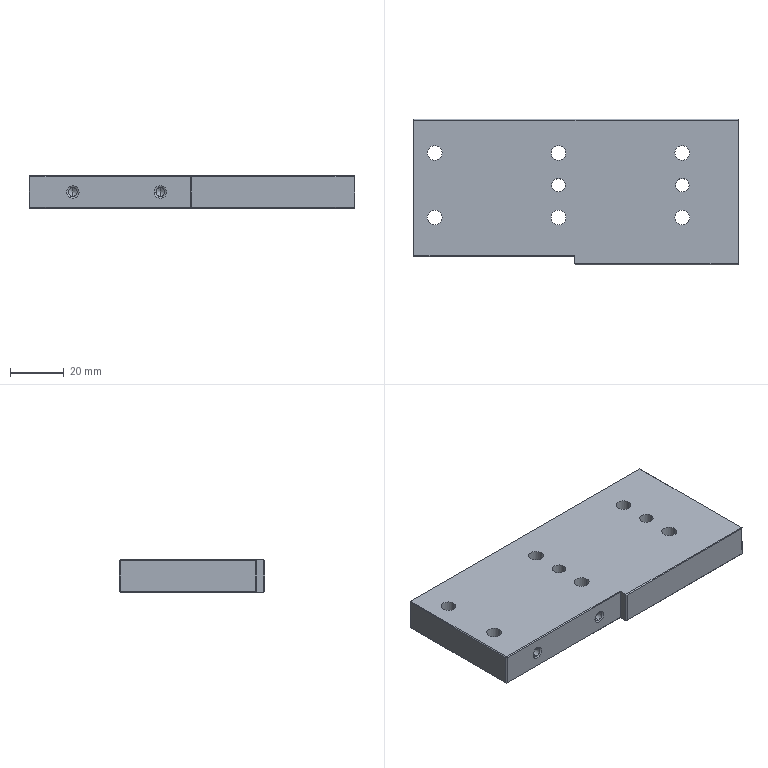Part | NX | 1 solid | 77 faces | box 121 x 54 x 12 mm | volume 71714 mm3 | cylinder 36 | plane 29 | cone 12 | commonest cylinder face diameters 5.5 x12 9.5 x12 3.3 x8 5 x4